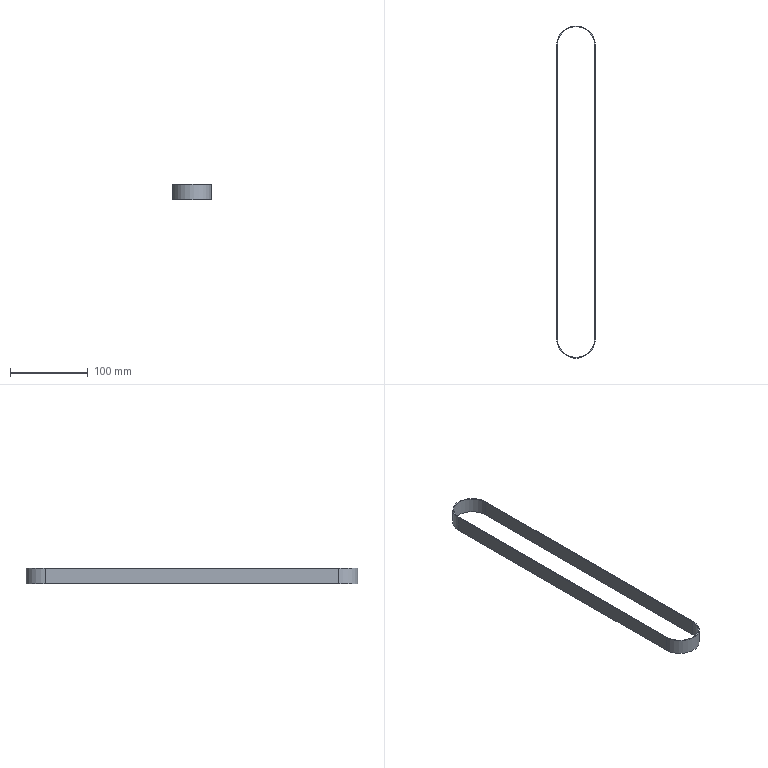Part | 1 solid | 10 faces | box 49.75 x 427.75 x 20 mm | volume 18183 mm3 | plane 6 | cylinder 4 | commonest cylinder face diameters 47.75 x2 49.75 x2
STEP:
#1=CARTESIAN_POINT('',(-24.875,378.,-10.));
#2=VERTEX_POINT('',#1);
#3=CARTESIAN_POINT('',(24.875,378.,-10.));
#4=VERTEX_POINT('',#3);
#5=CARTESIAN_POINT('',(0.,378.,-10.));
#6=DIRECTION('',(0.,0.,-1.));
#7=DIRECTION('',(-1.,0.,0.));
#8=AXIS2_PLACEMENT_3D('',#5,#6,#7);
#9=CIRCLE('',#8,24.875);
#10=EDGE_CURVE('',#2,#4,#9,.T.);
#11=ORIENTED_EDGE('',*,*,#10,.F.);
#12=CARTESIAN_POINT('',(-24.875,378.,10.));
#13=VERTEX_POINT('',#12);
#14=CARTESIAN_POINT('',(-24.875,378.,10.));
#15=DIRECTION('',(0.,0.,-1.));
#16=VECTOR('',#15,1000.);
#17=LINE('',#14,#16);
#18=EDGE_CURVE('',#13,#2,#17,.T.);
#19=ORIENTED_EDGE('',*,*,#18,.F.);
#20=CARTESIAN_POINT('',(24.875,378.,10.));
#21=VERTEX_POINT('',#20);
#22=CARTESIAN_POINT('',(0.,378.,10.));
#23=DIRECTION('',(0.,0.,-1.));
#24=DIRECTION('',(-1.,0.,0.));
#25=AXIS2_PLACEMENT_3D('',#22,#23,#24);
#26=CIRCLE('',#25,24.875);
#27=EDGE_CURVE('',#13,#21,#26,.T.);
#28=ORIENTED_EDGE('',*,*,#27,.T.);
#29=CARTESIAN_POINT('',(24.875,378.,10.));
#30=DIRECTION('',(0.,0.,-1.));
#31=VECTOR('',#30,1000.);
#32=LINE('',#29,#31);
#33=EDGE_CURVE('',#21,#4,#32,.T.);
#34=ORIENTED_EDGE('',*,*,#33,.T.);
#35=EDGE_LOOP('',(#11,#19,#28,#34));
#36=FACE_OUTER_BOUND('',#35,.T.);
#37=CARTESIAN_POINT('',(0.,378.,10.));
#38=DIRECTION('',(0.,0.,-1.));
#39=DIRECTION('',(-1.,0.,0.));
#40=AXIS2_PLACEMENT_3D('',#37,#38,#39);
#41=CYLINDRICAL_SURFACE('',#40,24.875);
#42=ADVANCED_FACE('',(#36),#41,.T.);
#43=CARTESIAN_POINT('',(-24.875,0.,-10.));
#44=VERTEX_POINT('',#43);
#45=CARTESIAN_POINT('',(-24.875,378.,-10.));
#46=DIRECTION('',(0.,1.,0.));
#47=VECTOR('',#46,1000.);
#48=LINE('',#45,#47);
#49=EDGE_CURVE('',#44,#2,#48,.T.);
#50=ORIENTED_EDGE('',*,*,#49,.F.);
#51=CARTESIAN_POINT('',(-24.875,0.,10.));
#52=VERTEX_POINT('',#51);
#53=CARTESIAN_POINT('',(-24.875,0.,10.));
#54=DIRECTION('',(0.,0.,-1.));
#55=VECTOR('',#54,1000.);
#56=LINE('',#53,#55);
#57=EDGE_CURVE('',#52,#44,#56,.T.);
#58=ORIENTED_EDGE('',*,*,#57,.F.);
#59=CARTESIAN_POINT('',(-24.875,378.,10.));
#60=DIRECTION('',(0.,1.,0.));
#61=VECTOR('',#60,1000.);
#62=LINE('',#59,#61);
#63=EDGE_CURVE('',#52,#13,#62,.T.);
#64=ORIENTED_EDGE('',*,*,#63,.T.);
#65=ORIENTED_EDGE('',*,*,#18,.T.);
#66=EDGE_LOOP('',(#50,#58,#64,#65));
#67=FACE_OUTER_BOUND('',#66,.T.);
#68=CARTESIAN_POINT('',(-24.875,378.,10.));
#69=DIRECTION('',(-1.,0.,0.));
#70=DIRECTION('',(0.,-1.,0.));
#71=AXIS2_PLACEMENT_3D('',#68,#69,#70);
#72=PLANE('',#71);
#73=ADVANCED_FACE('',(#67),#72,.T.);
#74=CARTESIAN_POINT('',(24.875,0.,-10.));
#75=VERTEX_POINT('',#74);
#76=CARTESIAN_POINT('',(0.,0.,-10.));
#77=DIRECTION('',(0.,0.,-1.));
#78=DIRECTION('',(-1.,0.,0.));
#79=AXIS2_PLACEMENT_3D('',#76,#77,#78);
#80=CIRCLE('',#79,24.875);
#81=EDGE_CURVE('',#75,#44,#80,.T.);
#82=ORIENTED_EDGE('',*,*,#81,.F.);
#83=CARTESIAN_POINT('',(24.875,0.,10.));
#84=VERTEX_POINT('',#83);
#85=CARTESIAN_POINT('',(24.875,0.,10.));
#86=DIRECTION('',(0.,0.,-1.));
#87=VECTOR('',#86,1000.);
#88=LINE('',#85,#87);
#89=EDGE_CURVE('',#84,#75,#88,.T.);
#90=ORIENTED_EDGE('',*,*,#89,.F.);
#91=CARTESIAN_POINT('',(0.,0.,10.));
#92=DIRECTION('',(0.,0.,-1.));
#93=DIRECTION('',(-1.,0.,0.));
#94=AXIS2_PLACEMENT_3D('',#91,#92,#93);
#95=CIRCLE('',#94,24.875);
#96=EDGE_CURVE('',#84,#52,#95,.T.);
#97=ORIENTED_EDGE('',*,*,#96,.T.);
#98=ORIENTED_EDGE('',*,*,#57,.T.);
#99=EDGE_LOOP('',(#82,#90,#97,#98));
#100=FACE_OUTER_BOUND('',#99,.T.);
#101=CARTESIAN_POINT('',(0.,0.,10.));
#102=DIRECTION('',(0.,0.,-1.));
#103=DIRECTION('',(-1.,0.,0.));
#104=AXIS2_PLACEMENT_3D('',#101,#102,#103);
#105=CYLINDRICAL_SURFACE('',#104,24.875);
#106=ADVANCED_FACE('',(#100),#105,.T.);
#107=CARTESIAN_POINT('',(24.875,378.,-10.));
#108=DIRECTION('',(0.,-1.,0.));
#109=VECTOR('',#108,1000.);
#110=LINE('',#107,#109);
#111=EDGE_CURVE('',#4,#75,#110,.T.);
#112=ORIENTED_EDGE('',*,*,#111,.F.);
#113=ORIENTED_EDGE('',*,*,#33,.F.);
#114=CARTESIAN_POINT('',(24.875,378.,10.));
#115=DIRECTION('',(0.,-1.,0.));
#116=VECTOR('',#115,1000.);
#117=LINE('',#114,#116);
#118=EDGE_CURVE('',#21,#84,#117,.T.);
#119=ORIENTED_EDGE('',*,*,#118,.T.);
#120=ORIENTED_EDGE('',*,*,#89,.T.);
#121=EDGE_LOOP('',(#112,#113,#119,#120));
#122=FACE_OUTER_BOUND('',#121,.T.);
#123=CARTESIAN_POINT('',(24.875,378.,10.));
#124=DIRECTION('',(1.,0.,0.));
#125=DIRECTION('',(0.,1.,0.));
#126=AXIS2_PLACEMENT_3D('',#123,#124,#125);
#127=PLANE('',#126);
#128=ADVANCED_FACE('',(#122),#127,.T.);
#129=CARTESIAN_POINT('',(-23.875,0.,10.));
#130=VERTEX_POINT('',#129);
#131=CARTESIAN_POINT('',(-23.875,378.,10.));
#132=VERTEX_POINT('',#131);
#133=CARTESIAN_POINT('',(-23.875,0.,10.));
#134=DIRECTION('',(0.,1.,0.));
#135=VECTOR('',#134,1000.);
#136=LINE('',#133,#135);
#137=EDGE_CURVE('',#130,#132,#136,.T.);
#138=ORIENTED_EDGE('',*,*,#137,.T.);
#139=CARTESIAN_POINT('',(23.875,378.,10.));
#140=VERTEX_POINT('',#139);
#141=CARTESIAN_POINT('',(0.,378.,10.));
#142=DIRECTION('',(0.,0.,-1.));
#143=DIRECTION('',(-1.,0.,0.));
#144=AXIS2_PLACEMENT_3D('',#141,#142,#143);
#145=CIRCLE('',#144,23.875);
#146=EDGE_CURVE('',#132,#140,#145,.T.);
#147=ORIENTED_EDGE('',*,*,#146,.T.);
#148=CARTESIAN_POINT('',(23.875,0.,10.));
#149=VERTEX_POINT('',#148);
#150=CARTESIAN_POINT('',(23.875,378.,10.));
#151=DIRECTION('',(0.,-1.,0.));
#152=VECTOR('',#151,1000.);
#153=LINE('',#150,#152);
#154=EDGE_CURVE('',#140,#149,#153,.T.);
#155=ORIENTED_EDGE('',*,*,#154,.T.);
#156=CARTESIAN_POINT('',(0.,0.,10.));
#157=DIRECTION('',(0.,0.,-1.));
#158=DIRECTION('',(-1.,0.,0.));
#159=AXIS2_PLACEMENT_3D('',#156,#157,#158);
#160=CIRCLE('',#159,23.875);
#161=EDGE_CURVE('',#149,#130,#160,.T.);
#162=ORIENTED_EDGE('',*,*,#161,.T.);
#163=EDGE_LOOP('',(#138,#147,#155,#162));
#164=FACE_BOUND('',#163,.T.);
#165=ORIENTED_EDGE('',*,*,#27,.F.);
#166=ORIENTED_EDGE('',*,*,#63,.F.);
#167=ORIENTED_EDGE('',*,*,#96,.F.);
#168=ORIENTED_EDGE('',*,*,#118,.F.);
#169=EDGE_LOOP('',(#165,#166,#167,#168));
#170=FACE_OUTER_BOUND('',#169,.T.);
#171=CARTESIAN_POINT('',(0.,378.,10.));
#172=DIRECTION('',(0.,0.,-1.));
#173=DIRECTION('',(-1.,0.,0.));
#174=AXIS2_PLACEMENT_3D('',#171,#172,#173);
#175=PLANE('',#174);
#176=ADVANCED_FACE('',(#164,#170),#175,.F.);
#177=CARTESIAN_POINT('',(-23.875,378.,-10.));
#178=VERTEX_POINT('',#177);
#179=CARTESIAN_POINT('',(23.875,378.,-10.));
#180=VERTEX_POINT('',#179);
#181=CARTESIAN_POINT('',(0.,378.,-10.));
#182=DIRECTION('',(0.,0.,-1.));
#183=DIRECTION('',(-1.,0.,0.));
#184=AXIS2_PLACEMENT_3D('',#181,#182,#183);
#185=CIRCLE('',#184,23.875);
#186=EDGE_CURVE('',#178,#180,#185,.T.);
#187=ORIENTED_EDGE('',*,*,#186,.F.);
#188=CARTESIAN_POINT('',(-23.875,0.,-10.));
#189=VERTEX_POINT('',#188);
#190=CARTESIAN_POINT('',(-23.875,0.,-10.));
#191=DIRECTION('',(0.,1.,0.));
#192=VECTOR('',#191,1000.);
#193=LINE('',#190,#192);
#194=EDGE_CURVE('',#189,#178,#193,.T.);
#195=ORIENTED_EDGE('',*,*,#194,.F.);
#196=CARTESIAN_POINT('',(23.875,0.,-10.));
#197=VERTEX_POINT('',#196);
#198=CARTESIAN_POINT('',(0.,0.,-10.));
#199=DIRECTION('',(0.,0.,-1.));
#200=DIRECTION('',(-1.,0.,0.));
#201=AXIS2_PLACEMENT_3D('',#198,#199,#200);
#202=CIRCLE('',#201,23.875);
#203=EDGE_CURVE('',#197,#189,#202,.T.);
#204=ORIENTED_EDGE('',*,*,#203,.F.);
#205=CARTESIAN_POINT('',(23.875,378.,-10.));
#206=DIRECTION('',(0.,-1.,0.));
#207=VECTOR('',#206,1000.);
#208=LINE('',#205,#207);
#209=EDGE_CURVE('',#180,#197,#208,.T.);
#210=ORIENTED_EDGE('',*,*,#209,.F.);
#211=EDGE_LOOP('',(#187,#195,#204,#210));
#212=FACE_BOUND('',#211,.T.);
#213=ORIENTED_EDGE('',*,*,#10,.T.);
#214=ORIENTED_EDGE('',*,*,#111,.T.);
#215=ORIENTED_EDGE('',*,*,#81,.T.);
#216=ORIENTED_EDGE('',*,*,#49,.T.);
#217=EDGE_LOOP('',(#213,#214,#215,#216));
#218=FACE_OUTER_BOUND('',#217,.T.);
#219=CARTESIAN_POINT('',(0.,378.,-10.));
#220=DIRECTION('',(0.,0.,-1.));
#221=DIRECTION('',(-1.,0.,0.));
#222=AXIS2_PLACEMENT_3D('',#219,#220,#221);
#223=PLANE('',#222);
#224=ADVANCED_FACE('',(#212,#218),#223,.T.);
#225=ORIENTED_EDGE('',*,*,#186,.T.);
#226=CARTESIAN_POINT('',(23.875,378.,10.));
#227=DIRECTION('',(0.,0.,-1.));
#228=VECTOR('',#227,1000.);
#229=LINE('',#226,#228);
#230=EDGE_CURVE('',#140,#180,#229,.T.);
#231=ORIENTED_EDGE('',*,*,#230,.F.);
#232=ORIENTED_EDGE('',*,*,#146,.F.);
#233=CARTESIAN_POINT('',(-23.875,378.,10.));
#234=DIRECTION('',(0.,0.,-1.));
#235=VECTOR('',#234,1000.);
#236=LINE('',#233,#235);
#237=EDGE_CURVE('',#132,#178,#236,.T.);
#238=ORIENTED_EDGE('',*,*,#237,.T.);
#239=EDGE_LOOP('',(#225,#231,#232,#238));
#240=FACE_OUTER_BOUND('',#239,.T.);
#241=CARTESIAN_POINT('',(0.,378.,10.));
#242=DIRECTION('',(0.,0.,-1.));
#243=DIRECTION('',(-1.,0.,0.));
#244=AXIS2_PLACEMENT_3D('',#241,#242,#243);
#245=CYLINDRICAL_SURFACE('',#244,23.875);
#246=ADVANCED_FACE('',(#240),#245,.F.);
#247=ORIENTED_EDGE('',*,*,#194,.T.);
#248=ORIENTED_EDGE('',*,*,#237,.F.);
#249=ORIENTED_EDGE('',*,*,#137,.F.);
#250=CARTESIAN_POINT('',(-23.875,0.,10.));
#251=DIRECTION('',(0.,0.,-1.));
#252=VECTOR('',#251,1000.);
#253=LINE('',#250,#252);
#254=EDGE_CURVE('',#130,#189,#253,.T.);
#255=ORIENTED_EDGE('',*,*,#254,.T.);
#256=EDGE_LOOP('',(#247,#248,#249,#255));
#257=FACE_OUTER_BOUND('',#256,.T.);
#258=CARTESIAN_POINT('',(-23.875,0.,10.));
#259=DIRECTION('',(-1.,0.,0.));
#260=DIRECTION('',(0.,-1.,0.));
#261=AXIS2_PLACEMENT_3D('',#258,#259,#260);
#262=PLANE('',#261);
#263=ADVANCED_FACE('',(#257),#262,.F.);
#264=ORIENTED_EDGE('',*,*,#203,.T.);
#265=ORIENTED_EDGE('',*,*,#254,.F.);
#266=ORIENTED_EDGE('',*,*,#161,.F.);
#267=CARTESIAN_POINT('',(23.875,0.,10.));
#268=DIRECTION('',(0.,0.,-1.));
#269=VECTOR('',#268,1000.);
#270=LINE('',#267,#269);
#271=EDGE_CURVE('',#149,#197,#270,.T.);
#272=ORIENTED_EDGE('',*,*,#271,.T.);
#273=EDGE_LOOP('',(#264,#265,#266,#272));
#274=FACE_OUTER_BOUND('',#273,.T.);
#275=CARTESIAN_POINT('',(0.,0.,10.));
#276=DIRECTION('',(0.,0.,-1.));
#277=DIRECTION('',(-1.,0.,0.));
#278=AXIS2_PLACEMENT_3D('',#275,#276,#277);
#279=CYLINDRICAL_SURFACE('',#278,23.875);
#280=ADVANCED_FACE('',(#274),#279,.F.);
#281=ORIENTED_EDGE('',*,*,#209,.T.);
#282=ORIENTED_EDGE('',*,*,#271,.F.);
#283=ORIENTED_EDGE('',*,*,#154,.F.);
#284=ORIENTED_EDGE('',*,*,#230,.T.);
#285=EDGE_LOOP('',(#281,#282,#283,#284));
#286=FACE_OUTER_BOUND('',#285,.T.);
#287=CARTESIAN_POINT('',(23.875,378.,10.));
#288=DIRECTION('',(1.,0.,0.));
#289=DIRECTION('',(0.,1.,0.));
#290=AXIS2_PLACEMENT_3D('',#287,#288,#289);
#291=PLANE('',#290);
#292=ADVANCED_FACE('',(#286),#291,.F.);
#293=CLOSED_SHELL('',(#42,#73,#106,#128,#176,#224,#246,#263,#280,#292));
#294=MANIFOLD_SOLID_BREP('',#293);
#295=CARTESIAN_POINT('',(0.,0.,0.));
#296=DIRECTION('',(0.,0.,1.));
#297=DIRECTION('',(1.,0.,0.));
#298=AXIS2_PLACEMENT_3D('',#295,#296,#297);
#299=(LENGTH_UNIT()NAMED_UNIT(*)SI_UNIT(.MILLI.,.METRE.));
#300=UNCERTAINTY_MEASURE_WITH_UNIT(LENGTH_MEASURE(0.00001),#299,'','');
#301=(NAMED_UNIT(*)PLANE_ANGLE_UNIT()SI_UNIT($,.RADIAN.));
#302=(NAMED_UNIT(*)SI_UNIT($,.STERADIAN.)SOLID_ANGLE_UNIT());
#303=(GEOMETRIC_REPRESENTATION_CONTEXT(3)GLOBAL_UNCERTAINTY_ASSIGNED_CONTEXT((#300))GLOBAL_UNIT_ASSIGNED_CONTEXT((#299,#301,#302))REPRESENTATION_CONTEXT('',''));
#304=ADVANCED_BREP_SHAPE_REPRESENTATION('',(#294,#298),#303);